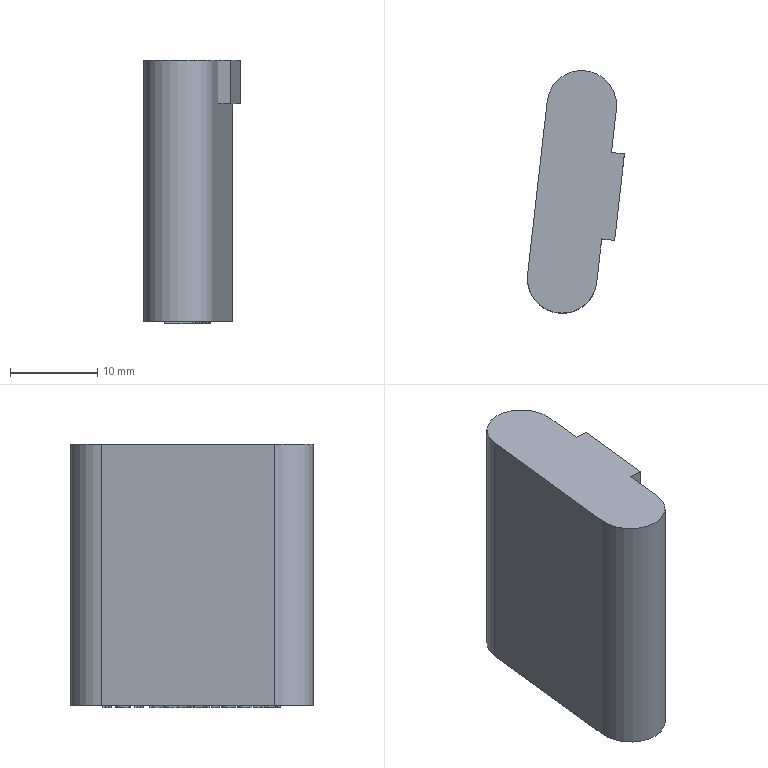Part | NX | features 13 2 | 1 solid | 113 faces | box 11.153 x 27.879 x 30.3 mm | volume 6390 mm3 | plane 94 | spline 17 | cylinder 2 | commonest cylinder face diameters 8 x2